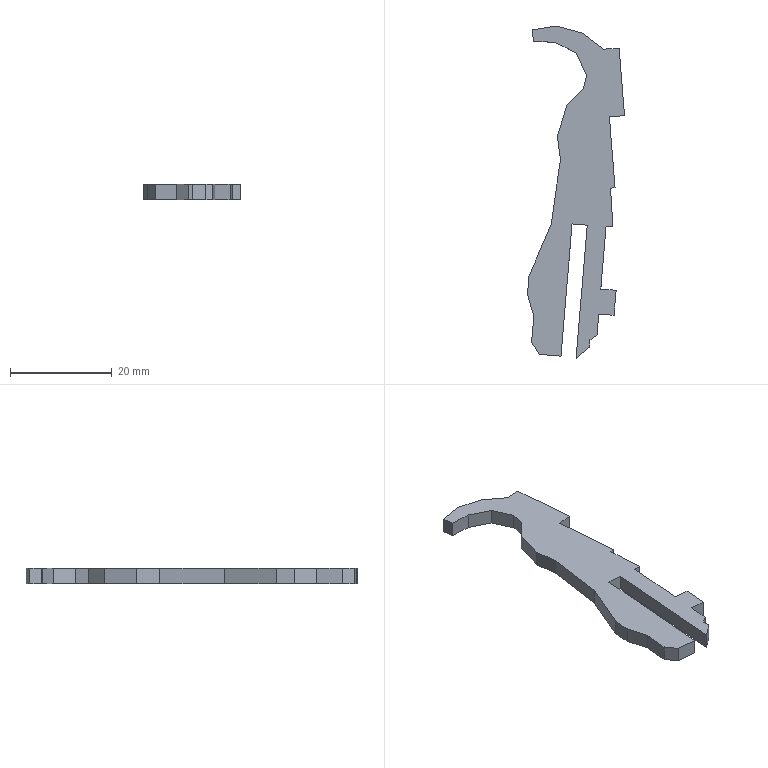Part | SolidWorks | features BaseBody 1 | 1 solid | 38 faces | box 19.065 x 65.26 x 3 mm | volume 1941 mm3 | plane 38
STEP:
#1=CARTESIAN_POINT('',(59.204,3.242,-1.5));
#2=VERTEX_POINT('',#1);
#3=CARTESIAN_POINT('',(60.084,3.312,-1.5));
#4=VERTEX_POINT('',#3);
#5=CARTESIAN_POINT('',(0.1171,-1.468,-1.5));
#6=DIRECTION('',(0.9968,0.07947,0.));
#7=VECTOR('',#6,1000.);
#8=LINE('',#5,#7);
#9=EDGE_CURVE('',#2,#4,#8,.T.);
#10=ORIENTED_EDGE('',*,*,#9,.F.);
#11=CARTESIAN_POINT('',(59.665,-4.354,-1.5));
#12=VERTEX_POINT('',#11);
#13=CARTESIAN_POINT('',(59.182,3.595,-1.5));
#14=DIRECTION('',(-0.06063,0.9982,0.));
#15=VECTOR('',#14,1000.);
#16=LINE('',#13,#15);
#17=EDGE_CURVE('',#12,#2,#16,.T.);
#18=ORIENTED_EDGE('',*,*,#17,.F.);
#19=CARTESIAN_POINT('',(58.319,-4.283,-1.5));
#20=VERTEX_POINT('',#19);
#21=CARTESIAN_POINT('',(-0.06393,-1.218,-1.5));
#22=DIRECTION('',(0.9986,-0.05243,0.));
#23=VECTOR('',#22,1000.);
#24=LINE('',#21,#23);
#25=EDGE_CURVE('',#20,#12,#24,.T.);
#26=ORIENTED_EDGE('',*,*,#25,.F.);
#27=CARTESIAN_POINT('',(57.287,-16.596,-1.5));
#28=VERTEX_POINT('',#27);
#29=CARTESIAN_POINT('',(58.268,-4.883,-1.5));
#30=DIRECTION('',(0.0835,0.9965,0.));
#31=VECTOR('',#30,1000.);
#32=LINE('',#29,#31);
#33=EDGE_CURVE('',#28,#20,#32,.T.);
#34=ORIENTED_EDGE('',*,*,#33,.F.);
#35=CARTESIAN_POINT('',(60.301,-16.848,-1.5));
#36=VERTEX_POINT('',#35);
#37=CARTESIAN_POINT('',(-0.9815,-11.713,-1.5));
#38=DIRECTION('',(-0.9965,0.0835,0.));
#39=VECTOR('',#38,1000.);
#40=LINE('',#37,#39);
#41=EDGE_CURVE('',#36,#28,#40,.T.);
#42=ORIENTED_EDGE('',*,*,#41,.F.);
#43=CARTESIAN_POINT('',(59.889,-21.763,-1.5));
#44=VERTEX_POINT('',#43);
#45=CARTESIAN_POINT('',(61.282,-5.135,-1.5));
#46=DIRECTION('',(0.0835,0.9965,0.));
#47=VECTOR('',#46,1000.);
#48=LINE('',#45,#47);
#49=EDGE_CURVE('',#44,#36,#48,.T.);
#50=ORIENTED_EDGE('',*,*,#49,.F.);
#51=CARTESIAN_POINT('',(56.875,-21.51,-1.5));
#52=VERTEX_POINT('',#51);
#53=CARTESIAN_POINT('',(-1.393,-16.627,-1.5));
#54=DIRECTION('',(0.9965,-0.0835,0.));
#55=VECTOR('',#54,1000.);
#56=LINE('',#53,#55);
#57=EDGE_CURVE('',#52,#44,#56,.T.);
#58=ORIENTED_EDGE('',*,*,#57,.F.);
#59=CARTESIAN_POINT('',(56.525,-25.691,-1.5));
#60=VERTEX_POINT('',#59);
#61=CARTESIAN_POINT('',(58.268,-4.883,-1.5));
#62=DIRECTION('',(0.0835,0.9965,0.));
#63=VECTOR('',#62,1000.);
#64=LINE('',#61,#63);
#65=EDGE_CURVE('',#60,#52,#64,.T.);
#66=ORIENTED_EDGE('',*,*,#65,.F.);
#67=CARTESIAN_POINT('',(55.154,-26.599,-1.5));
#68=VERTEX_POINT('',#67);
#69=CARTESIAN_POINT('',(29.095,-43.879,-1.5));
#70=DIRECTION('',(0.8334,0.5526,0.));
#71=VECTOR('',#70,1000.);
#72=LINE('',#69,#71);
#73=EDGE_CURVE('',#68,#60,#72,.T.);
#74=ORIENTED_EDGE('',*,*,#73,.F.);
#75=CARTESIAN_POINT('',(55.154,-28.004,-1.5));
#76=VERTEX_POINT('',#75);
#77=CARTESIAN_POINT('',(55.154,0.,-1.5));
#78=DIRECTION('',(0.,1.,0.));
#79=VECTOR('',#78,1000.);
#80=LINE('',#77,#79);
#81=EDGE_CURVE('',#76,#68,#80,.T.);
#82=ORIENTED_EDGE('',*,*,#81,.F.);
#83=CARTESIAN_POINT('',(52.433,-30.152,-1.5));
#84=VERTEX_POINT('',#83);
#85=CARTESIAN_POINT('',(34.797,-44.076,-1.5));
#86=DIRECTION('',(0.7849,0.6197,0.));
#87=VECTOR('',#86,1000.);
#88=LINE('',#85,#87);
#89=EDGE_CURVE('',#84,#76,#88,.T.);
#90=ORIENTED_EDGE('',*,*,#89,.F.);
#91=CARTESIAN_POINT('',(54.62,-4.056,-1.5));
#92=VERTEX_POINT('',#91);
#93=CARTESIAN_POINT('',(54.577,-4.573,-1.5));
#94=DIRECTION('',(-0.0835,-0.9965,0.));
#95=VECTOR('',#94,1000.);
#96=LINE('',#93,#95);
#97=EDGE_CURVE('',#92,#84,#96,.T.);
#98=ORIENTED_EDGE('',*,*,#97,.F.);
#99=CARTESIAN_POINT('',(51.63,-3.806,-1.5));
#100=VERTEX_POINT('',#99);
#101=CARTESIAN_POINT('',(0.04335,0.5173,-1.5));
#102=DIRECTION('',(0.9965,-0.0835,0.));
#103=VECTOR('',#102,1000.);
#104=LINE('',#101,#103);
#105=EDGE_CURVE('',#100,#92,#104,.T.);
#106=ORIENTED_EDGE('',*,*,#105,.F.);
#107=CARTESIAN_POINT('',(49.453,-29.79,-1.5));
#108=VERTEX_POINT('',#107);
#109=CARTESIAN_POINT('',(51.587,-4.323,-1.5));
#110=DIRECTION('',(0.0835,0.9965,0.));
#111=VECTOR('',#110,1000.);
#112=LINE('',#109,#111);
#113=EDGE_CURVE('',#108,#100,#112,.T.);
#114=ORIENTED_EDGE('',*,*,#113,.F.);
#115=CARTESIAN_POINT('',(45.268,-29.439,-1.5));
#116=VERTEX_POINT('',#115);
#117=CARTESIAN_POINT('',(-2.134,-25.467,-1.5));
#118=DIRECTION('',(0.9965,-0.0835,0.));
#119=VECTOR('',#118,1000.);
#120=LINE('',#117,#119);
#121=EDGE_CURVE('',#116,#108,#120,.T.);
#122=ORIENTED_EDGE('',*,*,#121,.F.);
#123=CARTESIAN_POINT('',(43.665,-27.089,-1.5));
#124=VERTEX_POINT('',#123);
#125=CARTESIAN_POINT('',(17.201,11.727,-1.5));
#126=DIRECTION('',(0.5633,-0.8262,0.));
#127=VECTOR('',#126,1000.);
#128=LINE('',#125,#127);
#129=EDGE_CURVE('',#124,#116,#128,.T.);
#130=ORIENTED_EDGE('',*,*,#129,.F.);
#131=CARTESIAN_POINT('',(44.13,-22.021,-1.5));
#132=VERTEX_POINT('',#131);
#133=CARTESIAN_POINT('',(45.764,-4.195,-1.5));
#134=DIRECTION('',(-0.09127,-0.9958,0.));
#135=VECTOR('',#134,1000.);
#136=LINE('',#133,#135);
#137=EDGE_CURVE('',#132,#124,#136,.T.);
#138=ORIENTED_EDGE('',*,*,#137,.F.);
#139=CARTESIAN_POINT('',(42.878,-17.641,-1.5));
#140=VERTEX_POINT('',#139);
#141=CARTESIAN_POINT('',(34.983,9.995,-1.5));
#142=DIRECTION('',(0.2747,-0.9615,0.));
#143=VECTOR('',#142,1000.);
#144=LINE('',#141,#143);
#145=EDGE_CURVE('',#140,#132,#144,.T.);
#146=ORIENTED_EDGE('',*,*,#145,.F.);
#147=CARTESIAN_POINT('',(43.161,-14.096,-1.5));
#148=VERTEX_POINT('',#147);
#149=CARTESIAN_POINT('',(44.005,-3.507,-1.5));
#150=DIRECTION('',(-0.07945,-0.9968,0.));
#151=VECTOR('',#150,1000.);
#152=LINE('',#149,#151);
#153=EDGE_CURVE('',#148,#140,#152,.T.);
#154=ORIENTED_EDGE('',*,*,#153,.F.);
#155=CARTESIAN_POINT('',(47.524,-3.891,-1.5));
#156=VERTEX_POINT('',#155);
#157=CARTESIAN_POINT('',(41.587,-17.778,-1.5));
#158=DIRECTION('',(-0.3931,-0.9195,0.));
#159=VECTOR('',#158,1000.);
#160=LINE('',#157,#159);
#161=EDGE_CURVE('',#156,#148,#160,.T.);
#162=ORIENTED_EDGE('',*,*,#161,.F.);
#163=CARTESIAN_POINT('',(49.355,8.81,-1.5));
#164=VERTEX_POINT('',#163);
#165=CARTESIAN_POINT('',(47.105,-6.792,-1.5));
#166=DIRECTION('',(-0.1427,-0.9898,0.));
#167=VECTOR('',#166,1000.);
#168=LINE('',#165,#167);
#169=EDGE_CURVE('',#164,#156,#168,.T.);
#170=ORIENTED_EDGE('',*,*,#169,.F.);
#171=CARTESIAN_POINT('',(48.752,13.356,-1.5));
#172=VERTEX_POINT('',#171);
#173=CARTESIAN_POINT('',(49.65,6.579,-1.5));
#174=DIRECTION('',(0.1314,-0.9913,0.));
#175=VECTOR('',#174,1000.);
#176=LINE('',#173,#175);
#177=EDGE_CURVE('',#172,#164,#176,.T.);
#178=ORIENTED_EDGE('',*,*,#177,.F.);
#179=CARTESIAN_POINT('',(50.657,19.656,-1.5));
#180=VERTEX_POINT('',#179);
#181=CARTESIAN_POINT('',(40.97,-12.386,-1.5));
#182=DIRECTION('',(-0.2894,-0.9572,0.));
#183=VECTOR('',#182,1000.);
#184=LINE('',#181,#183);
#185=EDGE_CURVE('',#180,#172,#184,.T.);
#186=ORIENTED_EDGE('',*,*,#185,.F.);
#187=CARTESIAN_POINT('',(53.865,22.82,-1.5));
#188=VERTEX_POINT('',#187);
#189=CARTESIAN_POINT('',(15.157,-15.365,-1.5));
#190=DIRECTION('',(-0.7119,-0.7023,0.));
#191=VECTOR('',#190,1000.);
#192=LINE('',#189,#191);
#193=EDGE_CURVE('',#188,#180,#192,.T.);
#194=ORIENTED_EDGE('',*,*,#193,.F.);
#195=CARTESIAN_POINT('',(54.479,25.44,-1.5));
#196=VERTEX_POINT('',#195);
#197=CARTESIAN_POINT('',(45.975,-10.791,-1.5));
#198=DIRECTION('',(-0.2285,-0.9735,0.));
#199=VECTOR('',#198,1000.);
#200=LINE('',#197,#199);
#201=EDGE_CURVE('',#196,#188,#200,.T.);
#202=ORIENTED_EDGE('',*,*,#201,.F.);
#203=CARTESIAN_POINT('',(52.51,29.78,-1.5));
#204=VERTEX_POINT('',#203);
#205=CARTESIAN_POINT('',(54.752,24.839,-1.5));
#206=DIRECTION('',(0.4131,-0.9107,0.));
#207=VECTOR('',#206,1000.);
#208=LINE('',#205,#207);
#209=EDGE_CURVE('',#204,#196,#208,.T.);
#210=ORIENTED_EDGE('',*,*,#209,.F.);
#211=CARTESIAN_POINT('',(48.197,31.904,-1.5));
#212=VERTEX_POINT('',#211);
#213=CARTESIAN_POINT('',(22.05,44.779,-1.5));
#214=DIRECTION('',(0.8971,-0.4418,0.));
#215=VECTOR('',#214,1000.);
#216=LINE('',#213,#215);
#217=EDGE_CURVE('',#212,#204,#216,.T.);
#218=ORIENTED_EDGE('',*,*,#217,.F.);
#219=CARTESIAN_POINT('',(44.079,32.075,-1.5));
#220=VERTEX_POINT('',#219);
#221=CARTESIAN_POINT('',(1.406,33.848,-1.5));
#222=DIRECTION('',(0.9991,-0.04151,0.));
#223=VECTOR('',#222,1000.);
#224=LINE('',#221,#223);
#225=EDGE_CURVE('',#220,#212,#224,.T.);
#226=ORIENTED_EDGE('',*,*,#225,.F.);
#227=CARTESIAN_POINT('',(43.773,34.357,-1.5));
#228=VERTEX_POINT('',#227);
#229=CARTESIAN_POINT('',(47.522,6.365,-1.5));
#230=DIRECTION('',(0.1327,-0.9912,0.));
#231=VECTOR('',#230,1000.);
#232=LINE('',#229,#231);
#233=EDGE_CURVE('',#228,#220,#232,.T.);
#234=ORIENTED_EDGE('',*,*,#233,.F.);
#235=CARTESIAN_POINT('',(48.53,35.108,-1.5));
#236=VERTEX_POINT('',#235);
#237=CARTESIAN_POINT('',(-4.228,26.779,-1.5));
#238=DIRECTION('',(-0.9878,-0.1559,0.));
#239=VECTOR('',#238,1000.);
#240=LINE('',#237,#239);
#241=EDGE_CURVE('',#236,#228,#240,.T.);
#242=ORIENTED_EDGE('',*,*,#241,.F.);
#243=CARTESIAN_POINT('',(53.668,33.7,-1.5));
#244=VERTEX_POINT('',#243);
#245=CARTESIAN_POINT('',(12.334,45.023,-1.5));
#246=DIRECTION('',(-0.9645,0.2642,0.));
#247=VECTOR('',#246,1000.);
#248=LINE('',#245,#247);
#249=EDGE_CURVE('',#244,#236,#248,.T.);
#250=ORIENTED_EDGE('',*,*,#249,.F.);
#251=CARTESIAN_POINT('',(57.888,30.559,-1.5));
#252=VERTEX_POINT('',#251);
#253=CARTESIAN_POINT('',(35.273,47.391,-1.5));
#254=DIRECTION('',(-0.8022,0.5971,0.));
#255=VECTOR('',#254,1000.);
#256=LINE('',#253,#255);
#257=EDGE_CURVE('',#252,#244,#256,.T.);
#258=ORIENTED_EDGE('',*,*,#257,.F.);
#259=CARTESIAN_POINT('',(60.888,30.739,-1.5));
#260=VERTEX_POINT('',#259);
#261=CARTESIAN_POINT('',(-1.617,26.995,-1.5));
#262=DIRECTION('',(-0.9982,-0.05979,0.));
#263=VECTOR('',#262,1000.);
#264=LINE('',#261,#263);
#265=EDGE_CURVE('',#260,#252,#264,.T.);
#266=ORIENTED_EDGE('',*,*,#265,.F.);
#267=CARTESIAN_POINT('',(61.944,17.486,-1.5));
#268=VERTEX_POINT('',#267);
#269=CARTESIAN_POINT('',(62.937,5.013,-1.5));
#270=DIRECTION('',(-0.0794,0.9968,0.));
#271=VECTOR('',#270,1000.);
#272=LINE('',#269,#271);
#273=EDGE_CURVE('',#268,#260,#272,.T.);
#274=ORIENTED_EDGE('',*,*,#273,.F.);
#275=CARTESIAN_POINT('',(58.973,17.249,-1.5));
#276=VERTEX_POINT('',#275);
#277=CARTESIAN_POINT('',(-0.9935,12.473,-1.5));
#278=DIRECTION('',(0.9968,0.0794,0.));
#279=VECTOR('',#278,1000.);
#280=LINE('',#277,#279);
#281=EDGE_CURVE('',#276,#268,#280,.T.);
#282=ORIENTED_EDGE('',*,*,#281,.F.);
#283=CARTESIAN_POINT('',(59.967,4.781,-1.5));
#284=DIRECTION('',(-0.07947,0.9968,0.));
#285=VECTOR('',#284,1000.);
#286=LINE('',#283,#285);
#287=EDGE_CURVE('',#4,#276,#286,.T.);
#288=ORIENTED_EDGE('',*,*,#287,.F.);
#289=EDGE_LOOP('',(#10,#18,#26,#34,#42,#50,#58,#66,#74,#82,#90,#98,#106,#114,#122,#130,#138,#146,#154,#162,#170,#178,#186,#194,#202,#210,#218,#226,#234,#242,#250,#258,#266,#274,#282,#288));
#290=FACE_OUTER_BOUND('',#289,.T.);
#291=CARTESIAN_POINT('',(0.,0.,-1.5));
#292=DIRECTION('',(0.,0.,1.));
#293=DIRECTION('',(1.,0.,0.));
#294=AXIS2_PLACEMENT_3D('',#291,#292,#293);
#295=PLANE('',#294);
#296=ADVANCED_FACE('',(#290),#295,.F.);
#297=CARTESIAN_POINT('',(59.204,3.242,1.5));
#298=VERTEX_POINT('',#297);
#299=CARTESIAN_POINT('',(60.084,3.312,1.5));
#300=VERTEX_POINT('',#299);
#301=CARTESIAN_POINT('',(0.1171,-1.468,1.5));
#302=DIRECTION('',(0.9968,0.07947,0.));
#303=VECTOR('',#302,1000.);
#304=LINE('',#301,#303);
#305=EDGE_CURVE('',#298,#300,#304,.T.);
#306=ORIENTED_EDGE('',*,*,#305,.T.);
#307=CARTESIAN_POINT('',(58.973,17.249,1.5));
#308=VERTEX_POINT('',#307);
#309=CARTESIAN_POINT('',(59.967,4.781,1.5));
#310=DIRECTION('',(-0.07947,0.9968,0.));
#311=VECTOR('',#310,1000.);
#312=LINE('',#309,#311);
#313=EDGE_CURVE('',#300,#308,#312,.T.);
#314=ORIENTED_EDGE('',*,*,#313,.T.);
#315=CARTESIAN_POINT('',(61.944,17.486,1.5));
#316=VERTEX_POINT('',#315);
#317=CARTESIAN_POINT('',(-0.9935,12.473,1.5));
#318=DIRECTION('',(0.9968,0.0794,0.));
#319=VECTOR('',#318,1000.);
#320=LINE('',#317,#319);
#321=EDGE_CURVE('',#308,#316,#320,.T.);
#322=ORIENTED_EDGE('',*,*,#321,.T.);
#323=CARTESIAN_POINT('',(60.888,30.739,1.5));
#324=VERTEX_POINT('',#323);
#325=CARTESIAN_POINT('',(62.937,5.013,1.5));
#326=DIRECTION('',(-0.0794,0.9968,0.));
#327=VECTOR('',#326,1000.);
#328=LINE('',#325,#327);
#329=EDGE_CURVE('',#316,#324,#328,.T.);
#330=ORIENTED_EDGE('',*,*,#329,.T.);
#331=CARTESIAN_POINT('',(57.888,30.559,1.5));
#332=VERTEX_POINT('',#331);
#333=CARTESIAN_POINT('',(-1.617,26.995,1.5));
#334=DIRECTION('',(-0.9982,-0.05979,0.));
#335=VECTOR('',#334,1000.);
#336=LINE('',#333,#335);
#337=EDGE_CURVE('',#324,#332,#336,.T.);
#338=ORIENTED_EDGE('',*,*,#337,.T.);
#339=CARTESIAN_POINT('',(53.668,33.7,1.5));
#340=VERTEX_POINT('',#339);
#341=CARTESIAN_POINT('',(35.273,47.391,1.5));
#342=DIRECTION('',(-0.8022,0.5971,0.));
#343=VECTOR('',#342,1000.);
#344=LINE('',#341,#343);
#345=EDGE_CURVE('',#332,#340,#344,.T.);
#346=ORIENTED_EDGE('',*,*,#345,.T.);
#347=CARTESIAN_POINT('',(48.53,35.108,1.5));
#348=VERTEX_POINT('',#347);
#349=CARTESIAN_POINT('',(12.334,45.023,1.5));
#350=DIRECTION('',(-0.9645,0.2642,0.));
#351=VECTOR('',#350,1000.);
#352=LINE('',#349,#351);
#353=EDGE_CURVE('',#340,#348,#352,.T.);
#354=ORIENTED_EDGE('',*,*,#353,.T.);
#355=CARTESIAN_POINT('',(43.773,34.357,1.5));
#356=VERTEX_POINT('',#355);
#357=CARTESIAN_POINT('',(-4.228,26.779,1.5));
#358=DIRECTION('',(-0.9878,-0.1559,0.));
#359=VECTOR('',#358,1000.);
#360=LINE('',#357,#359);
#361=EDGE_CURVE('',#348,#356,#360,.T.);
#362=ORIENTED_EDGE('',*,*,#361,.T.);
#363=CARTESIAN_POINT('',(44.079,32.075,1.5));
#364=VERTEX_POINT('',#363);
#365=CARTESIAN_POINT('',(47.522,6.365,1.5));
#366=DIRECTION('',(0.1327,-0.9912,0.));
#367=VECTOR('',#366,1000.);
#368=LINE('',#365,#367);
#369=EDGE_CURVE('',#356,#364,#368,.T.);
#370=ORIENTED_EDGE('',*,*,#369,.T.);
#371=CARTESIAN_POINT('',(48.197,31.904,1.5));
#372=VERTEX_POINT('',#371);
#373=CARTESIAN_POINT('',(1.406,33.848,1.5));
#374=DIRECTION('',(0.9991,-0.04151,0.));
#375=VECTOR('',#374,1000.);
#376=LINE('',#373,#375);
#377=EDGE_CURVE('',#364,#372,#376,.T.);
#378=ORIENTED_EDGE('',*,*,#377,.T.);
#379=CARTESIAN_POINT('',(52.51,29.78,1.5));
#380=VERTEX_POINT('',#379);
#381=CARTESIAN_POINT('',(22.05,44.779,1.5));
#382=DIRECTION('',(0.8971,-0.4418,0.));
#383=VECTOR('',#382,1000.);
#384=LINE('',#381,#383);
#385=EDGE_CURVE('',#372,#380,#384,.T.);
#386=ORIENTED_EDGE('',*,*,#385,.T.);
#387=CARTESIAN_POINT('',(54.479,25.44,1.5));
#388=VERTEX_POINT('',#387);
#389=CARTESIAN_POINT('',(54.752,24.839,1.5));
#390=DIRECTION('',(0.4131,-0.9107,0.));
#391=VECTOR('',#390,1000.);
#392=LINE('',#389,#391);
#393=EDGE_CURVE('',#380,#388,#392,.T.);
#394=ORIENTED_EDGE('',*,*,#393,.T.);
#395=CARTESIAN_POINT('',(53.865,22.82,1.5));
#396=VERTEX_POINT('',#395);
#397=CARTESIAN_POINT('',(45.975,-10.791,1.5));
#398=DIRECTION('',(-0.2285,-0.9735,0.));
#399=VECTOR('',#398,1000.);
#400=LINE('',#397,#399);
#401=EDGE_CURVE('',#388,#396,#400,.T.);
#402=ORIENTED_EDGE('',*,*,#401,.T.);
#403=CARTESIAN_POINT('',(50.657,19.656,1.5));
#404=VERTEX_POINT('',#403);
#405=CARTESIAN_POINT('',(15.157,-15.365,1.5));
#406=DIRECTION('',(-0.7119,-0.7023,0.));
#407=VECTOR('',#406,1000.);
#408=LINE('',#405,#407);
#409=EDGE_CURVE('',#396,#404,#408,.T.);
#410=ORIENTED_EDGE('',*,*,#409,.T.);
#411=CARTESIAN_POINT('',(48.752,13.356,1.5));
#412=VERTEX_POINT('',#411);
#413=CARTESIAN_POINT('',(40.97,-12.386,1.5));
#414=DIRECTION('',(-0.2894,-0.9572,0.));
#415=VECTOR('',#414,1000.);
#416=LINE('',#413,#415);
#417=EDGE_CURVE('',#404,#412,#416,.T.);
#418=ORIENTED_EDGE('',*,*,#417,.T.);
#419=CARTESIAN_POINT('',(49.355,8.81,1.5));
#420=VERTEX_POINT('',#419);
#421=CARTESIAN_POINT('',(49.65,6.579,1.5));
#422=DIRECTION('',(0.1314,-0.9913,0.));
#423=VECTOR('',#422,1000.);
#424=LINE('',#421,#423);
#425=EDGE_CURVE('',#412,#420,#424,.T.);
#426=ORIENTED_EDGE('',*,*,#425,.T.);
#427=CARTESIAN_POINT('',(47.524,-3.891,1.5));
#428=VERTEX_POINT('',#427);
#429=CARTESIAN_POINT('',(47.105,-6.792,1.5));
#430=DIRECTION('',(-0.1427,-0.9898,0.));
#431=VECTOR('',#430,1000.);
#432=LINE('',#429,#431);
#433=EDGE_CURVE('',#420,#428,#432,.T.);
#434=ORIENTED_EDGE('',*,*,#433,.T.);
#435=CARTESIAN_POINT('',(43.161,-14.096,1.5));
#436=VERTEX_POINT('',#435);
#437=CARTESIAN_POINT('',(41.587,-17.778,1.5));
#438=DIRECTION('',(-0.3931,-0.9195,0.));
#439=VECTOR('',#438,1000.);
#440=LINE('',#437,#439);
#441=EDGE_CURVE('',#428,#436,#440,.T.);
#442=ORIENTED_EDGE('',*,*,#441,.T.);
#443=CARTESIAN_POINT('',(42.878,-17.641,1.5));
#444=VERTEX_POINT('',#443);
#445=CARTESIAN_POINT('',(44.005,-3.507,1.5));
#446=DIRECTION('',(-0.07945,-0.9968,0.));
#447=VECTOR('',#446,1000.);
#448=LINE('',#445,#447);
#449=EDGE_CURVE('',#436,#444,#448,.T.);
#450=ORIENTED_EDGE('',*,*,#449,.T.);
#451=CARTESIAN_POINT('',(44.13,-22.021,1.5));
#452=VERTEX_POINT('',#451);
#453=CARTESIAN_POINT('',(34.983,9.995,1.5));
#454=DIRECTION('',(0.2747,-0.9615,0.));
#455=VECTOR('',#454,1000.);
#456=LINE('',#453,#455);
#457=EDGE_CURVE('',#444,#452,#456,.T.);
#458=ORIENTED_EDGE('',*,*,#457,.T.);
#459=CARTESIAN_POINT('',(43.665,-27.089,1.5));
#460=VERTEX_POINT('',#459);
#461=CARTESIAN_POINT('',(45.764,-4.195,1.5));
#462=DIRECTION('',(-0.09127,-0.9958,0.));
#463=VECTOR('',#462,1000.);
#464=LINE('',#461,#463);
#465=EDGE_CURVE('',#452,#460,#464,.T.);
#466=ORIENTED_EDGE('',*,*,#465,.T.);
#467=CARTESIAN_POINT('',(45.268,-29.439,1.5));
#468=VERTEX_POINT('',#467);
#469=CARTESIAN_POINT('',(17.201,11.727,1.5));
#470=DIRECTION('',(0.5633,-0.8262,0.));
#471=VECTOR('',#470,1000.);
#472=LINE('',#469,#471);
#473=EDGE_CURVE('',#460,#468,#472,.T.);
#474=ORIENTED_EDGE('',*,*,#473,.T.);
#475=CARTESIAN_POINT('',(49.453,-29.79,1.5));
#476=VERTEX_POINT('',#475);
#477=CARTESIAN_POINT('',(-2.134,-25.467,1.5));
#478=DIRECTION('',(0.9965,-0.0835,0.));
#479=VECTOR('',#478,1000.);
#480=LINE('',#477,#479);
#481=EDGE_CURVE('',#468,#476,#480,.T.);
#482=ORIENTED_EDGE('',*,*,#481,.T.);
#483=CARTESIAN_POINT('',(51.63,-3.806,1.5));
#484=VERTEX_POINT('',#483);
#485=CARTESIAN_POINT('',(51.587,-4.323,1.5));
#486=DIRECTION('',(0.0835,0.9965,0.));
#487=VECTOR('',#486,1000.);
#488=LINE('',#485,#487);
#489=EDGE_CURVE('',#476,#484,#488,.T.);
#490=ORIENTED_EDGE('',*,*,#489,.T.);
#491=CARTESIAN_POINT('',(54.62,-4.056,1.5));
#492=VERTEX_POINT('',#491);
#493=CARTESIAN_POINT('',(0.04335,0.5173,1.5));
#494=DIRECTION('',(0.9965,-0.0835,0.));
#495=VECTOR('',#494,1000.);
#496=LINE('',#493,#495);
#497=EDGE_CURVE('',#484,#492,#496,.T.);
#498=ORIENTED_EDGE('',*,*,#497,.T.);
#499=CARTESIAN_POINT('',(52.433,-30.152,1.5));
#500=VERTEX_POINT('',#499);
#501=CARTESIAN_POINT('',(54.577,-4.573,1.5));
#502=DIRECTION('',(-0.0835,-0.9965,0.));
#503=VECTOR('',#502,1000.);
#504=LINE('',#501,#503);
#505=EDGE_CURVE('',#492,#500,#504,.T.);
#506=ORIENTED_EDGE('',*,*,#505,.T.);
#507=CARTESIAN_POINT('',(55.154,-28.004,1.5));
#508=VERTEX_POINT('',#507);
#509=CARTESIAN_POINT('',(34.797,-44.076,1.5));
#510=DIRECTION('',(0.7849,0.6197,0.));
#511=VECTOR('',#510,1000.);
#512=LINE('',#509,#511);
#513=EDGE_CURVE('',#500,#508,#512,.T.);
#514=ORIENTED_EDGE('',*,*,#513,.T.);
#515=CARTESIAN_POINT('',(55.154,-26.599,1.5));
#516=VERTEX_POINT('',#515);
#517=CARTESIAN_POINT('',(55.154,0.,1.5));
#518=DIRECTION('',(0.,1.,0.));
#519=VECTOR('',#518,1000.);
#520=LINE('',#517,#519);
#521=EDGE_CURVE('',#508,#516,#520,.T.);
#522=ORIENTED_EDGE('',*,*,#521,.T.);
#523=CARTESIAN_POINT('',(56.525,-25.691,1.5));
#524=VERTEX_POINT('',#523);
#525=CARTESIAN_POINT('',(29.095,-43.879,1.5));
#526=DIRECTION('',(0.8334,0.5526,0.));
#527=VECTOR('',#526,1000.);
#528=LINE('',#525,#527);
#529=EDGE_CURVE('',#516,#524,#528,.T.);
#530=ORIENTED_EDGE('',*,*,#529,.T.);
#531=CARTESIAN_POINT('',(56.875,-21.51,1.5));
#532=VERTEX_POINT('',#531);
#533=CARTESIAN_POINT('',(58.268,-4.883,1.5));
#534=DIRECTION('',(0.0835,0.9965,0.));
#535=VECTOR('',#534,1000.);
#536=LINE('',#533,#535);
#537=EDGE_CURVE('',#524,#532,#536,.T.);
#538=ORIENTED_EDGE('',*,*,#537,.T.);
#539=CARTESIAN_POINT('',(59.889,-21.763,1.5));
#540=VERTEX_POINT('',#539);
#541=CARTESIAN_POINT('',(-1.393,-16.627,1.5));
#542=DIRECTION('',(0.9965,-0.0835,0.));
#543=VECTOR('',#542,1000.);
#544=LINE('',#541,#543);
#545=EDGE_CURVE('',#532,#540,#544,.T.);
#546=ORIENTED_EDGE('',*,*,#545,.T.);
#547=CARTESIAN_POINT('',(60.301,-16.848,1.5));
#548=VERTEX_POINT('',#547);
#549=CARTESIAN_POINT('',(61.282,-5.135,1.5));
#550=DIRECTION('',(0.0835,0.9965,0.));
#551=VECTOR('',#550,1000.);
#552=LINE('',#549,#551);
#553=EDGE_CURVE('',#540,#548,#552,.T.);
#554=ORIENTED_EDGE('',*,*,#553,.T.);
#555=CARTESIAN_POINT('',(57.287,-16.596,1.5));
#556=VERTEX_POINT('',#555);
#557=CARTESIAN_POINT('',(-0.9815,-11.713,1.5));
#558=DIRECTION('',(-0.9965,0.0835,0.));
#559=VECTOR('',#558,1000.);
#560=LINE('',#557,#559);
#561=EDGE_CURVE('',#548,#556,#560,.T.);
#562=ORIENTED_EDGE('',*,*,#561,.T.);
#563=CARTESIAN_POINT('',(58.319,-4.283,1.5));
#564=VERTEX_POINT('',#563);
#565=CARTESIAN_POINT('',(58.268,-4.883,1.5));
#566=DIRECTION('',(0.0835,0.9965,0.));
#567=VECTOR('',#566,1000.);
#568=LINE('',#565,#567);
#569=EDGE_CURVE('',#556,#564,#568,.T.);
#570=ORIENTED_EDGE('',*,*,#569,.T.);
#571=CARTESIAN_POINT('',(59.665,-4.354,1.5));
#572=VERTEX_POINT('',#571);
#573=CARTESIAN_POINT('',(-0.06393,-1.218,1.5));
#574=DIRECTION('',(0.9986,-0.05243,0.));
#575=VECTOR('',#574,1000.);
#576=LINE('',#573,#575);
#577=EDGE_CURVE('',#564,#572,#576,.T.);
#578=ORIENTED_EDGE('',*,*,#577,.T.);
#579=CARTESIAN_POINT('',(59.182,3.595,1.5));
#580=DIRECTION('',(-0.06063,0.9982,0.));
#581=VECTOR('',#580,1000.);
#582=LINE('',#579,#581);
#583=EDGE_CURVE('',#572,#298,#582,.T.);
#584=ORIENTED_EDGE('',*,*,#583,.T.);
#585=EDGE_LOOP('',(#306,#314,#322,#330,#338,#346,#354,#362,#370,#378,#386,#394,#402,#410,#418,#426,#434,#442,#450,#458,#466,#474,#482,#490,#498,#506,#514,#522,#530,#538,#546,#554,#562,#570,#578,#584));
#586=FACE_OUTER_BOUND('',#585,.T.);
#587=CARTESIAN_POINT('',(0.,0.,1.5));
#588=DIRECTION('',(0.,0.,1.));
#589=DIRECTION('',(1.,0.,0.));
#590=AXIS2_PLACEMENT_3D('',#587,#588,#589);
#591=PLANE('',#590);
#592=ADVANCED_FACE('',(#586),#591,.T.);
#593=ORIENTED_EDGE('',*,*,#17,.T.);
#594=CARTESIAN_POINT('',(59.204,3.242,1.5));
#595=DIRECTION('',(0.,0.,-1.));
#596=VECTOR('',#595,1000.);
#597=LINE('',#594,#596);
#598=EDGE_CURVE('',#298,#2,#597,.T.);
#599=ORIENTED_EDGE('',*,*,#598,.F.);
#600=ORIENTED_EDGE('',*,*,#583,.F.);
#601=CARTESIAN_POINT('',(59.665,-4.354,1.5));
#602=DIRECTION('',(0.,0.,-1.));
#603=VECTOR('',#602,1000.);
#604=LINE('',#601,#603);
#605=EDGE_CURVE('',#572,#12,#604,.T.);
#606=ORIENTED_EDGE('',*,*,#605,.T.);
#607=EDGE_LOOP('',(#593,#599,#600,#606));
#608=FACE_OUTER_BOUND('',#607,.T.);
#609=CARTESIAN_POINT('',(59.182,3.595,1.5));
#610=DIRECTION('',(-0.9982,-0.06063,0.));
#611=DIRECTION('',(-0.06063,0.9982,0.));
#612=AXIS2_PLACEMENT_3D('',#609,#610,#611);
#613=PLANE('',#612);
#614=ADVANCED_FACE('',(#608),#613,.F.);
#615=ORIENTED_EDGE('',*,*,#25,.T.);
#616=ORIENTED_EDGE('',*,*,#605,.F.);
#617=ORIENTED_EDGE('',*,*,#577,.F.);
#618=CARTESIAN_POINT('',(58.319,-4.283,1.5));
#619=DIRECTION('',(0.,0.,-1.));
#620=VECTOR('',#619,1000.);
#621=LINE('',#618,#620);
#622=EDGE_CURVE('',#564,#20,#621,.T.);
#623=ORIENTED_EDGE('',*,*,#622,.T.);
#624=EDGE_LOOP('',(#615,#616,#617,#623));
#625=FACE_OUTER_BOUND('',#624,.T.);
#626=CARTESIAN_POINT('',(-0.06393,-1.218,1.5));
#627=DIRECTION('',(0.05243,0.9986,0.));
#628=DIRECTION('',(0.,0.,-1.));
#629=AXIS2_PLACEMENT_3D('',#626,#627,#628);
#630=PLANE('',#629);
#631=ADVANCED_FACE('',(#625),#630,.F.);
#632=ORIENTED_EDGE('',*,*,#33,.T.);
#633=ORIENTED_EDGE('',*,*,#622,.F.);
#634=ORIENTED_EDGE('',*,*,#569,.F.);
#635=CARTESIAN_POINT('',(57.287,-16.596,1.5));
#636=DIRECTION('',(0.,0.,-1.));
#637=VECTOR('',#636,1000.);
#638=LINE('',#635,#637);
#639=EDGE_CURVE('',#556,#28,#638,.T.);
#640=ORIENTED_EDGE('',*,*,#639,.T.);
#641=EDGE_LOOP('',(#632,#633,#634,#640));
#642=FACE_OUTER_BOUND('',#641,.T.);
#643=CARTESIAN_POINT('',(58.268,-4.883,1.5));
#644=DIRECTION('',(-0.9965,0.0835,0.));
#645=DIRECTION('',(0.,0.,1.));
#646=AXIS2_PLACEMENT_3D('',#643,#644,#645);
#647=PLANE('',#646);
#648=ADVANCED_FACE('',(#642),#647,.F.);
#649=ORIENTED_EDGE('',*,*,#41,.T.);
#650=ORIENTED_EDGE('',*,*,#639,.F.);
#651=ORIENTED_EDGE('',*,*,#561,.F.);
#652=CARTESIAN_POINT('',(60.301,-16.848,1.5));
#653=DIRECTION('',(0.,0.,-1.));
#654=VECTOR('',#653,1000.);
#655=LINE('',#652,#654);
#656=EDGE_CURVE('',#548,#36,#655,.T.);
#657=ORIENTED_EDGE('',*,*,#656,.T.);
#658=EDGE_LOOP('',(#649,#650,#651,#657));
#659=FACE_OUTER_BOUND('',#658,.T.);
#660=CARTESIAN_POINT('',(-0.9815,-11.713,1.5));
#661=DIRECTION('',(-0.0835,-0.9965,0.));
#662=DIRECTION('',(-0.9965,0.0835,0.));
#663=AXIS2_PLACEMENT_3D('',#660,#661,#662);
#664=PLANE('',#663);
#665=ADVANCED_FACE('',(#659),#664,.F.);
#666=ORIENTED_EDGE('',*,*,#49,.T.);
#667=ORIENTED_EDGE('',*,*,#656,.F.);
#668=ORIENTED_EDGE('',*,*,#553,.F.);
#669=CARTESIAN_POINT('',(59.889,-21.763,1.5));
#670=DIRECTION('',(0.,0.,-1.));
#671=VECTOR('',#670,1000.);
#672=LINE('',#669,#671);
#673=EDGE_CURVE('',#540,#44,#672,.T.);
#674=ORIENTED_EDGE('',*,*,#673,.T.);
#675=EDGE_LOOP('',(#666,#667,#668,#674));
#676=FACE_OUTER_BOUND('',#675,.T.);
#677=CARTESIAN_POINT('',(61.282,-5.135,1.5));
#678=DIRECTION('',(-0.9965,0.0835,0.));
#679=DIRECTION('',(0.,0.,1.));
#680=AXIS2_PLACEMENT_3D('',#677,#678,#679);
#681=PLANE('',#680);
#682=ADVANCED_FACE('',(#676),#681,.F.);
#683=ORIENTED_EDGE('',*,*,#57,.T.);
#684=ORIENTED_EDGE('',*,*,#673,.F.);
#685=ORIENTED_EDGE('',*,*,#545,.F.);
#686=CARTESIAN_POINT('',(56.875,-21.51,1.5));
#687=DIRECTION('',(0.,0.,-1.));
#688=VECTOR('',#687,1000.);
#689=LINE('',#686,#688);
#690=EDGE_CURVE('',#532,#52,#689,.T.);
#691=ORIENTED_EDGE('',*,*,#690,.T.);
#692=EDGE_LOOP('',(#683,#684,#685,#691));
#693=FACE_OUTER_BOUND('',#692,.T.);
#694=CARTESIAN_POINT('',(-1.393,-16.627,1.5));
#695=DIRECTION('',(0.0835,0.9965,0.));
#696=DIRECTION('',(0.,0.,-1.));
#697=AXIS2_PLACEMENT_3D('',#694,#695,#696);
#698=PLANE('',#697);
#699=ADVANCED_FACE('',(#693),#698,.F.);
#700=ORIENTED_EDGE('',*,*,#65,.T.);
#701=ORIENTED_EDGE('',*,*,#690,.F.);
#702=ORIENTED_EDGE('',*,*,#537,.F.);
#703=CARTESIAN_POINT('',(56.525,-25.691,1.5));
#704=DIRECTION('',(0.,0.,-1.));
#705=VECTOR('',#704,1000.);
#706=LINE('',#703,#705);
#707=EDGE_CURVE('',#524,#60,#706,.T.);
#708=ORIENTED_EDGE('',*,*,#707,.T.);
#709=EDGE_LOOP('',(#700,#701,#702,#708));
#710=FACE_OUTER_BOUND('',#709,.T.);
#711=CARTESIAN_POINT('',(58.268,-4.883,1.5));
#712=DIRECTION('',(-0.9965,0.0835,0.));
#713=DIRECTION('',(0.,0.,1.));
#714=AXIS2_PLACEMENT_3D('',#711,#712,#713);
#715=PLANE('',#714);
#716=ADVANCED_FACE('',(#710),#715,.F.);
#717=ORIENTED_EDGE('',*,*,#73,.T.);
#718=ORIENTED_EDGE('',*,*,#707,.F.);
#719=ORIENTED_EDGE('',*,*,#529,.F.);
#720=CARTESIAN_POINT('',(55.154,-26.599,1.5));
#721=DIRECTION('',(0.,0.,-1.));
#722=VECTOR('',#721,1000.);
#723=LINE('',#720,#722);
#724=EDGE_CURVE('',#516,#68,#723,.T.);
#725=ORIENTED_EDGE('',*,*,#724,.T.);
#726=EDGE_LOOP('',(#717,#718,#719,#725));
#727=FACE_OUTER_BOUND('',#726,.T.);
#728=CARTESIAN_POINT('',(29.095,-43.879,1.5));
#729=DIRECTION('',(-0.5526,0.8334,0.));
#730=DIRECTION('',(0.,0.,1.));
#731=AXIS2_PLACEMENT_3D('',#728,#729,#730);
#732=PLANE('',#731);
#733=ADVANCED_FACE('',(#727),#732,.F.);
#734=ORIENTED_EDGE('',*,*,#81,.T.);
#735=ORIENTED_EDGE('',*,*,#724,.F.);
#736=ORIENTED_EDGE('',*,*,#521,.F.);
#737=CARTESIAN_POINT('',(55.154,-28.004,1.5));
#738=DIRECTION('',(0.,0.,-1.));
#739=VECTOR('',#738,1000.);
#740=LINE('',#737,#739);
#741=EDGE_CURVE('',#508,#76,#740,.T.);
#742=ORIENTED_EDGE('',*,*,#741,.T.);
#743=EDGE_LOOP('',(#734,#735,#736,#742));
#744=FACE_OUTER_BOUND('',#743,.T.);
#745=CARTESIAN_POINT('',(55.154,0.,1.5));
#746=DIRECTION('',(-1.,0.,0.));
#747=DIRECTION('',(0.,0.,1.));
#748=AXIS2_PLACEMENT_3D('',#745,#746,#747);
#749=PLANE('',#748);
#750=ADVANCED_FACE('',(#744),#749,.F.);
#751=ORIENTED_EDGE('',*,*,#89,.T.);
#752=ORIENTED_EDGE('',*,*,#741,.F.);
#753=ORIENTED_EDGE('',*,*,#513,.F.);
#754=CARTESIAN_POINT('',(52.433,-30.152,1.5));
#755=DIRECTION('',(0.,0.,-1.));
#756=VECTOR('',#755,1000.);
#757=LINE('',#754,#756);
#758=EDGE_CURVE('',#500,#84,#757,.T.);
#759=ORIENTED_EDGE('',*,*,#758,.T.);
#760=EDGE_LOOP('',(#751,#752,#753,#759));
#761=FACE_OUTER_BOUND('',#760,.T.);
#762=CARTESIAN_POINT('',(34.797,-44.076,1.5));
#763=DIRECTION('',(-0.6197,0.7849,0.));
#764=DIRECTION('',(0.,0.,1.));
#765=AXIS2_PLACEMENT_3D('',#762,#763,#764);
#766=PLANE('',#765);
#767=ADVANCED_FACE('',(#761),#766,.F.);
#768=ORIENTED_EDGE('',*,*,#97,.T.);
#769=ORIENTED_EDGE('',*,*,#758,.F.);
#770=ORIENTED_EDGE('',*,*,#505,.F.);
#771=CARTESIAN_POINT('',(54.62,-4.056,1.5));
#772=DIRECTION('',(0.,0.,-1.));
#773=VECTOR('',#772,1000.);
#774=LINE('',#771,#773);
#775=EDGE_CURVE('',#492,#92,#774,.T.);
#776=ORIENTED_EDGE('',*,*,#775,.T.);
#777=EDGE_LOOP('',(#768,#769,#770,#776));
#778=FACE_OUTER_BOUND('',#777,.T.);
#779=CARTESIAN_POINT('',(54.577,-4.573,1.5));
#780=DIRECTION('',(0.9965,-0.0835,0.));
#781=DIRECTION('',(0.,0.,-1.));
#782=AXIS2_PLACEMENT_3D('',#779,#780,#781);
#783=PLANE('',#782);
#784=ADVANCED_FACE('',(#778),#783,.F.);
#785=ORIENTED_EDGE('',*,*,#105,.T.);
#786=ORIENTED_EDGE('',*,*,#775,.F.);
#787=ORIENTED_EDGE('',*,*,#497,.F.);
#788=CARTESIAN_POINT('',(51.63,-3.806,1.5));
#789=DIRECTION('',(0.,0.,-1.));
#790=VECTOR('',#789,1000.);
#791=LINE('',#788,#790);
#792=EDGE_CURVE('',#484,#100,#791,.T.);
#793=ORIENTED_EDGE('',*,*,#792,.T.);
#794=EDGE_LOOP('',(#785,#786,#787,#793));
#795=FACE_OUTER_BOUND('',#794,.T.);
#796=CARTESIAN_POINT('',(0.04335,0.5173,1.5));
#797=DIRECTION('',(0.0835,0.9965,0.));
#798=DIRECTION('',(0.,0.,-1.));
#799=AXIS2_PLACEMENT_3D('',#796,#797,#798);
#800=PLANE('',#799);
#801=ADVANCED_FACE('',(#795),#800,.F.);
#802=ORIENTED_EDGE('',*,*,#113,.T.);
#803=ORIENTED_EDGE('',*,*,#792,.F.);
#804=ORIENTED_EDGE('',*,*,#489,.F.);
#805=CARTESIAN_POINT('',(49.453,-29.79,1.5));
#806=DIRECTION('',(0.,0.,-1.));
#807=VECTOR('',#806,1000.);
#808=LINE('',#805,#807);
#809=EDGE_CURVE('',#476,#108,#808,.T.);
#810=ORIENTED_EDGE('',*,*,#809,.T.);
#811=EDGE_LOOP('',(#802,#803,#804,#810));
#812=FACE_OUTER_BOUND('',#811,.T.);
#813=CARTESIAN_POINT('',(51.587,-4.323,1.5));
#814=DIRECTION('',(-0.9965,0.0835,0.));
#815=DIRECTION('',(0.,0.,1.));
#816=AXIS2_PLACEMENT_3D('',#813,#814,#815);
#817=PLANE('',#816);
#818=ADVANCED_FACE('',(#812),#817,.F.);
#819=ORIENTED_EDGE('',*,*,#121,.T.);
#820=ORIENTED_EDGE('',*,*,#809,.F.);
#821=ORIENTED_EDGE('',*,*,#481,.F.);
#822=CARTESIAN_POINT('',(45.268,-29.439,1.5));
#823=DIRECTION('',(0.,0.,-1.));
#824=VECTOR('',#823,1000.);
#825=LINE('',#822,#824);
#826=EDGE_CURVE('',#468,#116,#825,.T.);
#827=ORIENTED_EDGE('',*,*,#826,.T.);
#828=EDGE_LOOP('',(#819,#820,#821,#827));
#829=FACE_OUTER_BOUND('',#828,.T.);
#830=CARTESIAN_POINT('',(-2.134,-25.467,1.5));
#831=DIRECTION('',(0.0835,0.9965,0.));
#832=DIRECTION('',(0.,0.,-1.));
#833=AXIS2_PLACEMENT_3D('',#830,#831,#832);
#834=PLANE('',#833);
#835=ADVANCED_FACE('',(#829),#834,.F.);
#836=ORIENTED_EDGE('',*,*,#129,.T.);
#837=ORIENTED_EDGE('',*,*,#826,.F.);
#838=ORIENTED_EDGE('',*,*,#473,.F.);
#839=CARTESIAN_POINT('',(43.665,-27.089,1.5));
#840=DIRECTION('',(0.,0.,-1.));
#841=VECTOR('',#840,1000.);
#842=LINE('',#839,#841);
#843=EDGE_CURVE('',#460,#124,#842,.T.);
#844=ORIENTED_EDGE('',*,*,#843,.T.);
#845=EDGE_LOOP('',(#836,#837,#838,#844));
#846=FACE_OUTER_BOUND('',#845,.T.);
#847=CARTESIAN_POINT('',(17.201,11.727,1.5));
#848=DIRECTION('',(0.8262,0.5633,0.));
#849=DIRECTION('',(0.,0.,-1.));
#850=AXIS2_PLACEMENT_3D('',#847,#848,#849);
#851=PLANE('',#850);
#852=ADVANCED_FACE('',(#846),#851,.F.);
#853=ORIENTED_EDGE('',*,*,#137,.T.);
#854=ORIENTED_EDGE('',*,*,#843,.F.);
#855=ORIENTED_EDGE('',*,*,#465,.F.);
#856=CARTESIAN_POINT('',(44.13,-22.021,1.5));
#857=DIRECTION('',(0.,0.,-1.));
#858=VECTOR('',#857,1000.);
#859=LINE('',#856,#858);
#860=EDGE_CURVE('',#452,#132,#859,.T.);
#861=ORIENTED_EDGE('',*,*,#860,.T.);
#862=EDGE_LOOP('',(#853,#854,#855,#861));
#863=FACE_OUTER_BOUND('',#862,.T.);
#864=CARTESIAN_POINT('',(45.764,-4.195,1.5));
#865=DIRECTION('',(0.9958,-0.09127,0.));
#866=DIRECTION('',(0.,0.,-1.));
#867=AXIS2_PLACEMENT_3D('',#864,#865,#866);
#868=PLANE('',#867);
#869=ADVANCED_FACE('',(#863),#868,.F.);
#870=ORIENTED_EDGE('',*,*,#145,.T.);
#871=ORIENTED_EDGE('',*,*,#860,.F.);
#872=ORIENTED_EDGE('',*,*,#457,.F.);
#873=CARTESIAN_POINT('',(42.878,-17.641,1.5));
#874=DIRECTION('',(0.,0.,-1.));
#875=VECTOR('',#874,1000.);
#876=LINE('',#873,#875);
#877=EDGE_CURVE('',#444,#140,#876,.T.);
#878=ORIENTED_EDGE('',*,*,#877,.T.);
#879=EDGE_LOOP('',(#870,#871,#872,#878));
#880=FACE_OUTER_BOUND('',#879,.T.);
#881=CARTESIAN_POINT('',(34.983,9.995,1.5));
#882=DIRECTION('',(0.9615,0.2747,0.));
#883=DIRECTION('',(0.,0.,-1.));
#884=AXIS2_PLACEMENT_3D('',#881,#882,#883);
#885=PLANE('',#884);
#886=ADVANCED_FACE('',(#880),#885,.F.);
#887=ORIENTED_EDGE('',*,*,#153,.T.);
#888=ORIENTED_EDGE('',*,*,#877,.F.);
#889=ORIENTED_EDGE('',*,*,#449,.F.);
#890=CARTESIAN_POINT('',(43.161,-14.096,1.5));
#891=DIRECTION('',(0.,0.,-1.));
#892=VECTOR('',#891,1000.);
#893=LINE('',#890,#892);
#894=EDGE_CURVE('',#436,#148,#893,.T.);
#895=ORIENTED_EDGE('',*,*,#894,.T.);
#896=EDGE_LOOP('',(#887,#888,#889,#895));
#897=FACE_OUTER_BOUND('',#896,.T.);
#898=CARTESIAN_POINT('',(44.005,-3.507,1.5));
#899=DIRECTION('',(0.9968,-0.07945,0.));
#900=DIRECTION('',(0.,0.,-1.));
#901=AXIS2_PLACEMENT_3D('',#898,#899,#900);
#902=PLANE('',#901);
#903=ADVANCED_FACE('',(#897),#902,.F.);
#904=ORIENTED_EDGE('',*,*,#161,.T.);
#905=ORIENTED_EDGE('',*,*,#894,.F.);
#906=ORIENTED_EDGE('',*,*,#441,.F.);
#907=CARTESIAN_POINT('',(47.524,-3.891,1.5));
#908=DIRECTION('',(0.,0.,-1.));
#909=VECTOR('',#908,1000.);
#910=LINE('',#907,#909);
#911=EDGE_CURVE('',#428,#156,#910,.T.);
#912=ORIENTED_EDGE('',*,*,#911,.T.);
#913=EDGE_LOOP('',(#904,#905,#906,#912));
#914=FACE_OUTER_BOUND('',#913,.T.);
#915=CARTESIAN_POINT('',(41.587,-17.778,1.5));
#916=DIRECTION('',(0.9195,-0.3931,0.));
#917=DIRECTION('',(0.,0.,-1.));
#918=AXIS2_PLACEMENT_3D('',#915,#916,#917);
#919=PLANE('',#918);
#920=ADVANCED_FACE('',(#914),#919,.F.);
#921=ORIENTED_EDGE('',*,*,#169,.T.);
#922=ORIENTED_EDGE('',*,*,#911,.F.);
#923=ORIENTED_EDGE('',*,*,#433,.F.);
#924=CARTESIAN_POINT('',(49.355,8.81,1.5));
#925=DIRECTION('',(0.,0.,-1.));
#926=VECTOR('',#925,1000.);
#927=LINE('',#924,#926);
#928=EDGE_CURVE('',#420,#164,#927,.T.);
#929=ORIENTED_EDGE('',*,*,#928,.T.);
#930=EDGE_LOOP('',(#921,#922,#923,#929));
#931=FACE_OUTER_BOUND('',#930,.T.);
#932=CARTESIAN_POINT('',(47.105,-6.792,1.5));
#933=DIRECTION('',(0.9898,-0.1427,0.));
#934=DIRECTION('',(0.,0.,-1.));
#935=AXIS2_PLACEMENT_3D('',#932,#933,#934);
#936=PLANE('',#935);
#937=ADVANCED_FACE('',(#931),#936,.F.);
#938=ORIENTED_EDGE('',*,*,#177,.T.);
#939=ORIENTED_EDGE('',*,*,#928,.F.);
#940=ORIENTED_EDGE('',*,*,#425,.F.);
#941=CARTESIAN_POINT('',(48.752,13.356,1.5));
#942=DIRECTION('',(0.,0.,-1.));
#943=VECTOR('',#942,1000.);
#944=LINE('',#941,#943);
#945=EDGE_CURVE('',#412,#172,#944,.T.);
#946=ORIENTED_EDGE('',*,*,#945,.T.);
#947=EDGE_LOOP('',(#938,#939,#940,#946));
#948=FACE_OUTER_BOUND('',#947,.T.);
#949=CARTESIAN_POINT('',(49.65,6.579,1.5));
#950=DIRECTION('',(0.9913,0.1314,0.));
#951=DIRECTION('',(0.,0.,-1.));
#952=AXIS2_PLACEMENT_3D('',#949,#950,#951);
#953=PLANE('',#952);
#954=ADVANCED_FACE('',(#948),#953,.F.);
#955=ORIENTED_EDGE('',*,*,#185,.T.);
#956=ORIENTED_EDGE('',*,*,#945,.F.);
#957=ORIENTED_EDGE('',*,*,#417,.F.);
#958=CARTESIAN_POINT('',(50.657,19.656,1.5));
#959=DIRECTION('',(0.,0.,-1.));
#960=VECTOR('',#959,1000.);
#961=LINE('',#958,#960);
#962=EDGE_CURVE('',#404,#180,#961,.T.);
#963=ORIENTED_EDGE('',*,*,#962,.T.);
#964=EDGE_LOOP('',(#955,#956,#957,#963));
#965=FACE_OUTER_BOUND('',#964,.T.);
#966=CARTESIAN_POINT('',(40.97,-12.386,1.5));
#967=DIRECTION('',(0.9572,-0.2894,0.));
#968=DIRECTION('',(0.,0.,-1.));
#969=AXIS2_PLACEMENT_3D('',#966,#967,#968);
#970=PLANE('',#969);
#971=ADVANCED_FACE('',(#965),#970,.F.);
#972=ORIENTED_EDGE('',*,*,#193,.T.);
#973=ORIENTED_EDGE('',*,*,#962,.F.);
#974=ORIENTED_EDGE('',*,*,#409,.F.);
#975=CARTESIAN_POINT('',(53.865,22.82,1.5));
#976=DIRECTION('',(0.,0.,-1.));
#977=VECTOR('',#976,1000.);
#978=LINE('',#975,#977);
#979=EDGE_CURVE('',#396,#188,#978,.T.);
#980=ORIENTED_EDGE('',*,*,#979,.T.);
#981=EDGE_LOOP('',(#972,#973,#974,#980));
#982=FACE_OUTER_BOUND('',#981,.T.);
#983=CARTESIAN_POINT('',(15.157,-15.365,1.5));
#984=DIRECTION('',(0.7023,-0.7119,0.));
#985=DIRECTION('',(0.,0.,-1.));
#986=AXIS2_PLACEMENT_3D('',#983,#984,#985);
#987=PLANE('',#986);
#988=ADVANCED_FACE('',(#982),#987,.F.);
#989=ORIENTED_EDGE('',*,*,#201,.T.);
#990=ORIENTED_EDGE('',*,*,#979,.F.);
#991=ORIENTED_EDGE('',*,*,#401,.F.);
#992=CARTESIAN_POINT('',(54.479,25.44,1.5));
#993=DIRECTION('',(0.,0.,-1.));
#994=VECTOR('',#993,1000.);
#995=LINE('',#992,#994);
#996=EDGE_CURVE('',#388,#196,#995,.T.);
#997=ORIENTED_EDGE('',*,*,#996,.T.);
#998=EDGE_LOOP('',(#989,#990,#991,#997));
#999=FACE_OUTER_BOUND('',#998,.T.);
#1000=CARTESIAN_POINT('',(45.975,-10.791,1.5));
#1001=DIRECTION('',(0.9735,-0.2285,0.));
#1002=DIRECTION('',(0.,0.,-1.));
#1003=AXIS2_PLACEMENT_3D('',#1000,#1001,#1002);
#1004=PLANE('',#1003);
#1005=ADVANCED_FACE('',(#999),#1004,.F.);
#1006=ORIENTED_EDGE('',*,*,#209,.T.);
#1007=ORIENTED_EDGE('',*,*,#996,.F.);
#1008=ORIENTED_EDGE('',*,*,#393,.F.);
#1009=CARTESIAN_POINT('',(52.51,29.78,1.5));
#1010=DIRECTION('',(0.,0.,-1.));
#1011=VECTOR('',#1010,1000.);
#1012=LINE('',#1009,#1011);
#1013=EDGE_CURVE('',#380,#204,#1012,.T.);
#1014=ORIENTED_EDGE('',*,*,#1013,.T.);
#1015=EDGE_LOOP('',(#1006,#1007,#1008,#1014));
#1016=FACE_OUTER_BOUND('',#1015,.T.);
#1017=CARTESIAN_POINT('',(54.752,24.839,1.5));
#1018=DIRECTION('',(0.9107,0.4131,0.));
#1019=DIRECTION('',(0.,0.,-1.));
#1020=AXIS2_PLACEMENT_3D('',#1017,#1018,#1019);
#1021=PLANE('',#1020);
#1022=ADVANCED_FACE('',(#1016),#1021,.F.);
#1023=ORIENTED_EDGE('',*,*,#217,.T.);
#1024=ORIENTED_EDGE('',*,*,#1013,.F.);
#1025=ORIENTED_EDGE('',*,*,#385,.F.);
#1026=CARTESIAN_POINT('',(48.197,31.904,1.5));
#1027=DIRECTION('',(0.,0.,-1.));
#1028=VECTOR('',#1027,1000.);
#1029=LINE('',#1026,#1028);
#1030=EDGE_CURVE('',#372,#212,#1029,.T.);
#1031=ORIENTED_EDGE('',*,*,#1030,.T.);
#1032=EDGE_LOOP('',(#1023,#1024,#1025,#1031));
#1033=FACE_OUTER_BOUND('',#1032,.T.);
#1034=CARTESIAN_POINT('',(22.05,44.779,1.5));
#1035=DIRECTION('',(0.4418,0.8971,0.));
#1036=DIRECTION('',(0.,0.,-1.));
#1037=AXIS2_PLACEMENT_3D('',#1034,#1035,#1036);
#1038=PLANE('',#1037);
#1039=ADVANCED_FACE('',(#1033),#1038,.F.);
#1040=ORIENTED_EDGE('',*,*,#225,.T.);
#1041=ORIENTED_EDGE('',*,*,#1030,.F.);
#1042=ORIENTED_EDGE('',*,*,#377,.F.);
#1043=CARTESIAN_POINT('',(44.079,32.075,1.5));
#1044=DIRECTION('',(0.,0.,-1.));
#1045=VECTOR('',#1044,1000.);
#1046=LINE('',#1043,#1045);
#1047=EDGE_CURVE('',#364,#220,#1046,.T.);
#1048=ORIENTED_EDGE('',*,*,#1047,.T.);
#1049=EDGE_LOOP('',(#1040,#1041,#1042,#1048));
#1050=FACE_OUTER_BOUND('',#1049,.T.);
#1051=CARTESIAN_POINT('',(1.406,33.848,1.5));
#1052=DIRECTION('',(0.04151,0.9991,0.));
#1053=DIRECTION('',(0.,0.,-1.));
#1054=AXIS2_PLACEMENT_3D('',#1051,#1052,#1053);
#1055=PLANE('',#1054);
#1056=ADVANCED_FACE('',(#1050),#1055,.F.);
#1057=ORIENTED_EDGE('',*,*,#233,.T.);
#1058=ORIENTED_EDGE('',*,*,#1047,.F.);
#1059=ORIENTED_EDGE('',*,*,#369,.F.);
#1060=CARTESIAN_POINT('',(43.773,34.357,1.5));
#1061=DIRECTION('',(0.,0.,-1.));
#1062=VECTOR('',#1061,1000.);
#1063=LINE('',#1060,#1062);
#1064=EDGE_CURVE('',#356,#228,#1063,.T.);
#1065=ORIENTED_EDGE('',*,*,#1064,.T.);
#1066=EDGE_LOOP('',(#1057,#1058,#1059,#1065));
#1067=FACE_OUTER_BOUND('',#1066,.T.);
#1068=CARTESIAN_POINT('',(47.522,6.365,1.5));
#1069=DIRECTION('',(0.9912,0.1327,0.));
#1070=DIRECTION('',(0.,0.,-1.));
#1071=AXIS2_PLACEMENT_3D('',#1068,#1069,#1070);
#1072=PLANE('',#1071);
#1073=ADVANCED_FACE('',(#1067),#1072,.F.);
#1074=ORIENTED_EDGE('',*,*,#241,.T.);
#1075=ORIENTED_EDGE('',*,*,#1064,.F.);
#1076=ORIENTED_EDGE('',*,*,#361,.F.);
#1077=CARTESIAN_POINT('',(48.53,35.108,1.5));
#1078=DIRECTION('',(0.,0.,-1.));
#1079=VECTOR('',#1078,1000.);
#1080=LINE('',#1077,#1079);
#1081=EDGE_CURVE('',#348,#236,#1080,.T.);
#1082=ORIENTED_EDGE('',*,*,#1081,.T.);
#1083=EDGE_LOOP('',(#1074,#1075,#1076,#1082));
#1084=FACE_OUTER_BOUND('',#1083,.T.);
#1085=CARTESIAN_POINT('',(-4.228,26.779,1.5));
#1086=DIRECTION('',(0.1559,-0.9878,0.));
#1087=DIRECTION('',(0.,0.,-1.));
#1088=AXIS2_PLACEMENT_3D('',#1085,#1086,#1087);
#1089=PLANE('',#1088);
#1090=ADVANCED_FACE('',(#1084),#1089,.F.);
#1091=ORIENTED_EDGE('',*,*,#249,.T.);
#1092=ORIENTED_EDGE('',*,*,#1081,.F.);
#1093=ORIENTED_EDGE('',*,*,#353,.F.);
#1094=CARTESIAN_POINT('',(53.668,33.7,1.5));
#1095=DIRECTION('',(0.,0.,-1.));
#1096=VECTOR('',#1095,1000.);
#1097=LINE('',#1094,#1096);
#1098=EDGE_CURVE('',#340,#244,#1097,.T.);
#1099=ORIENTED_EDGE('',*,*,#1098,.T.);
#1100=EDGE_LOOP('',(#1091,#1092,#1093,#1099));
#1101=FACE_OUTER_BOUND('',#1100,.T.);
#1102=CARTESIAN_POINT('',(12.334,45.023,1.5));
#1103=DIRECTION('',(-0.2642,-0.9645,0.));
#1104=DIRECTION('',(-0.9645,0.2642,0.));
#1105=AXIS2_PLACEMENT_3D('',#1102,#1103,#1104);
#1106=PLANE('',#1105);
#1107=ADVANCED_FACE('',(#1101),#1106,.F.);
#1108=ORIENTED_EDGE('',*,*,#257,.T.);
#1109=ORIENTED_EDGE('',*,*,#1098,.F.);
#1110=ORIENTED_EDGE('',*,*,#345,.F.);
#1111=CARTESIAN_POINT('',(57.888,30.559,1.5));
#1112=DIRECTION('',(0.,0.,-1.));
#1113=VECTOR('',#1112,1000.);
#1114=LINE('',#1111,#1113);
#1115=EDGE_CURVE('',#332,#252,#1114,.T.);
#1116=ORIENTED_EDGE('',*,*,#1115,.T.);
#1117=EDGE_LOOP('',(#1108,#1109,#1110,#1116));
#1118=FACE_OUTER_BOUND('',#1117,.T.);
#1119=CARTESIAN_POINT('',(35.273,47.391,1.5));
#1120=DIRECTION('',(-0.5971,-0.8022,0.));
#1121=DIRECTION('',(-0.8022,0.5971,0.));
#1122=AXIS2_PLACEMENT_3D('',#1119,#1120,#1121);
#1123=PLANE('',#1122);
#1124=ADVANCED_FACE('',(#1118),#1123,.F.);
#1125=ORIENTED_EDGE('',*,*,#265,.T.);
#1126=ORIENTED_EDGE('',*,*,#1115,.F.);
#1127=ORIENTED_EDGE('',*,*,#337,.F.);
#1128=CARTESIAN_POINT('',(60.888,30.739,1.5));
#1129=DIRECTION('',(0.,0.,-1.));
#1130=VECTOR('',#1129,1000.);
#1131=LINE('',#1128,#1130);
#1132=EDGE_CURVE('',#324,#260,#1131,.T.);
#1133=ORIENTED_EDGE('',*,*,#1132,.T.);
#1134=EDGE_LOOP('',(#1125,#1126,#1127,#1133));
#1135=FACE_OUTER_BOUND('',#1134,.T.);
#1136=CARTESIAN_POINT('',(-1.617,26.995,1.5));
#1137=DIRECTION('',(0.05979,-0.9982,0.));
#1138=DIRECTION('',(0.,0.,-1.));
#1139=AXIS2_PLACEMENT_3D('',#1136,#1137,#1138);
#1140=PLANE('',#1139);
#1141=ADVANCED_FACE('',(#1135),#1140,.F.);
#1142=ORIENTED_EDGE('',*,*,#273,.T.);
#1143=ORIENTED_EDGE('',*,*,#1132,.F.);
#1144=ORIENTED_EDGE('',*,*,#329,.F.);
#1145=CARTESIAN_POINT('',(61.944,17.486,1.5));
#1146=DIRECTION('',(0.,0.,-1.));
#1147=VECTOR('',#1146,1000.);
#1148=LINE('',#1145,#1147);
#1149=EDGE_CURVE('',#316,#268,#1148,.T.);
#1150=ORIENTED_EDGE('',*,*,#1149,.T.);
#1151=EDGE_LOOP('',(#1142,#1143,#1144,#1150));
#1152=FACE_OUTER_BOUND('',#1151,.T.);
#1153=CARTESIAN_POINT('',(62.937,5.013,1.5));
#1154=DIRECTION('',(-0.9968,-0.0794,0.));
#1155=DIRECTION('',(-0.0794,0.9968,0.));
#1156=AXIS2_PLACEMENT_3D('',#1153,#1154,#1155);
#1157=PLANE('',#1156);
#1158=ADVANCED_FACE('',(#1152),#1157,.F.);
#1159=ORIENTED_EDGE('',*,*,#281,.T.);
#1160=ORIENTED_EDGE('',*,*,#1149,.F.);
#1161=ORIENTED_EDGE('',*,*,#321,.F.);
#1162=CARTESIAN_POINT('',(58.973,17.249,1.5));
#1163=DIRECTION('',(0.,0.,-1.));
#1164=VECTOR('',#1163,1000.);
#1165=LINE('',#1162,#1164);
#1166=EDGE_CURVE('',#308,#276,#1165,.T.);
#1167=ORIENTED_EDGE('',*,*,#1166,.T.);
#1168=EDGE_LOOP('',(#1159,#1160,#1161,#1167));
#1169=FACE_OUTER_BOUND('',#1168,.T.);
#1170=CARTESIAN_POINT('',(-0.9935,12.473,1.5));
#1171=DIRECTION('',(-0.0794,0.9968,0.));
#1172=DIRECTION('',(0.,0.,1.));
#1173=AXIS2_PLACEMENT_3D('',#1170,#1171,#1172);
#1174=PLANE('',#1173);
#1175=ADVANCED_FACE('',(#1169),#1174,.F.);
#1176=ORIENTED_EDGE('',*,*,#287,.T.);
#1177=ORIENTED_EDGE('',*,*,#1166,.F.);
#1178=ORIENTED_EDGE('',*,*,#313,.F.);
#1179=CARTESIAN_POINT('',(60.084,3.312,1.5));
#1180=DIRECTION('',(0.,0.,-1.));
#1181=VECTOR('',#1180,1000.);
#1182=LINE('',#1179,#1181);
#1183=EDGE_CURVE('',#300,#4,#1182,.T.);
#1184=ORIENTED_EDGE('',*,*,#1183,.T.);
#1185=EDGE_LOOP('',(#1176,#1177,#1178,#1184));
#1186=FACE_OUTER_BOUND('',#1185,.T.);
#1187=CARTESIAN_POINT('',(59.967,4.781,1.5));
#1188=DIRECTION('',(-0.9968,-0.07947,0.));
#1189=DIRECTION('',(-0.07947,0.9968,0.));
#1190=AXIS2_PLACEMENT_3D('',#1187,#1188,#1189);
#1191=PLANE('',#1190);
#1192=ADVANCED_FACE('',(#1186),#1191,.F.);
#1193=ORIENTED_EDGE('',*,*,#9,.T.);
#1194=ORIENTED_EDGE('',*,*,#1183,.F.);
#1195=ORIENTED_EDGE('',*,*,#305,.F.);
#1196=ORIENTED_EDGE('',*,*,#598,.T.);
#1197=EDGE_LOOP('',(#1193,#1194,#1195,#1196));
#1198=FACE_OUTER_BOUND('',#1197,.T.);
#1199=CARTESIAN_POINT('',(0.1171,-1.468,1.5));
#1200=DIRECTION('',(-0.07947,0.9968,0.));
#1201=DIRECTION('',(0.,0.,1.));
#1202=AXIS2_PLACEMENT_3D('',#1199,#1200,#1201);
#1203=PLANE('',#1202);
#1204=ADVANCED_FACE('',(#1198),#1203,.F.);
#1205=CLOSED_SHELL('',(#296,#592,#614,#631,#648,#665,#682,#699,#716,#733,#750,#767,#784,#801,#818,#835,#852,#869,#886,#903,#920,#937,#954,#971,#988,#1005,#1022,#1039,#1056,#1073,#1090,#1107,#1124,#1141,#1158,#1175,#1192,#1204));
#1206=MANIFOLD_SOLID_BREP('',#1205);
#1207=CARTESIAN_POINT('',(0.,0.,0.));
#1208=DIRECTION('',(0.,0.,1.));
#1209=DIRECTION('',(1.,0.,0.));
#1210=AXIS2_PLACEMENT_3D('',#1207,#1208,#1209);
#1211=(LENGTH_UNIT()NAMED_UNIT(*)SI_UNIT(.MILLI.,.METRE.));
#1212=UNCERTAINTY_MEASURE_WITH_UNIT(LENGTH_MEASURE(0.00001),#1211,'','');
#1213=(NAMED_UNIT(*)PLANE_ANGLE_UNIT()SI_UNIT($,.RADIAN.));
#1214=(NAMED_UNIT(*)SI_UNIT($,.STERADIAN.)SOLID_ANGLE_UNIT());
#1215=(GEOMETRIC_REPRESENTATION_CONTEXT(3)GLOBAL_UNCERTAINTY_ASSIGNED_CONTEXT((#1212))GLOBAL_UNIT_ASSIGNED_CONTEXT((#1211,#1213,#1214))REPRESENTATION_CONTEXT('',''));
#1216=ADVANCED_BREP_SHAPE_REPRESENTATION('',(#1206,#1210),#1215);